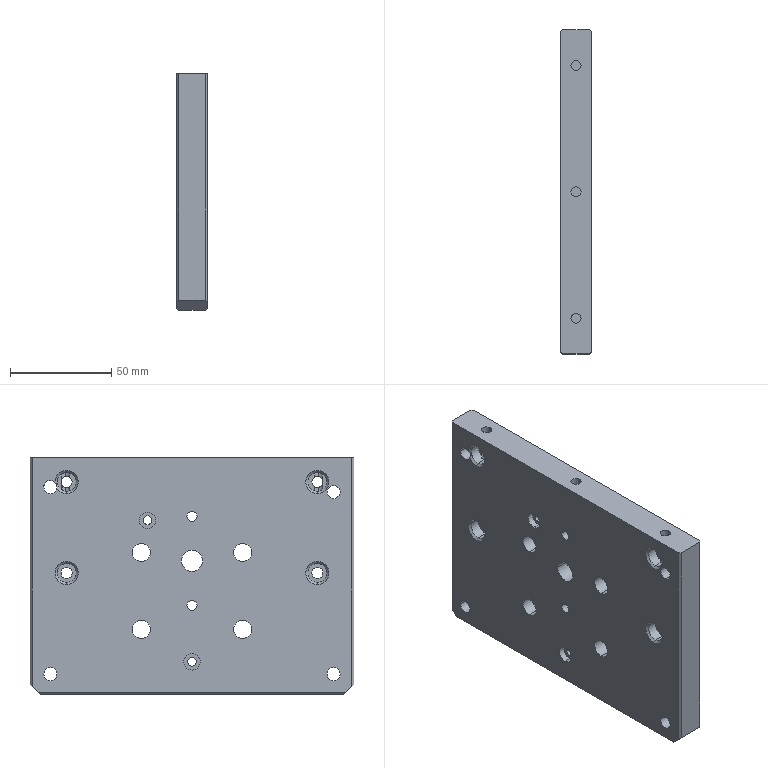Part | STEP file | PN_0008 | 1 solid | 101 faces | box 15 x 160 x 117 mm | volume 266376 mm3 | cylinder 60 | plane 28 | cone 13 | commonest cylinder face diameters 5 x12 5.5 x9 6.5 x8 9 x8 9.5 x8 12 x5